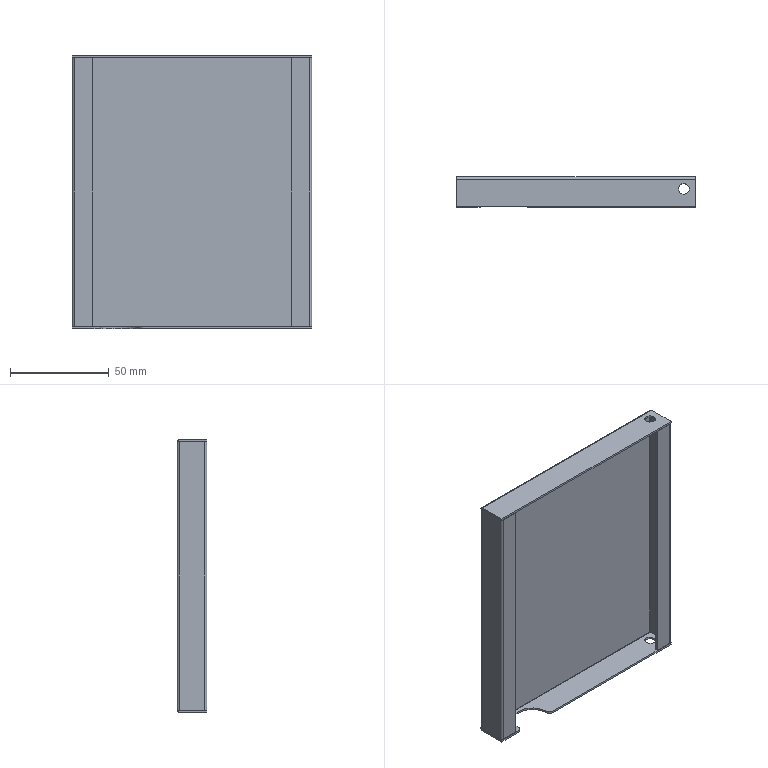Part | STEP file | 鼠标盖Plate-01^TY.NE-0002-01-015A 鼠标盖Plate-dddeger | 1 solid | 66 faces | box 121 x 15 x 138 mm | volume 25843 mm3 | plane 47 | cylinder 19 | commonest cylinder face diameters 0.4 x6 2.4 x6 5.4 x4 4 x2 20 x1